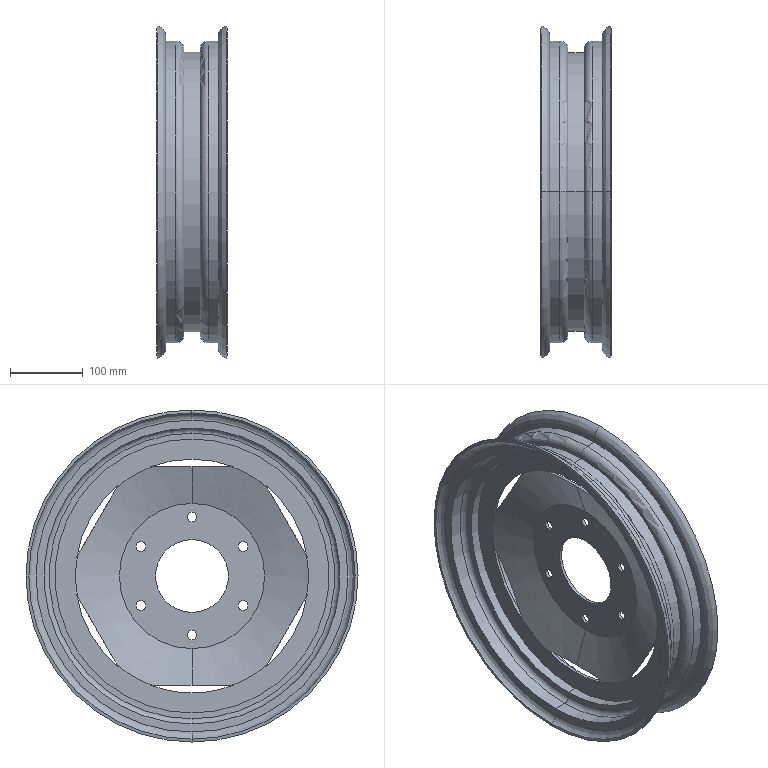Part | SolidWorks | 1 solid | 79 faces | box 96.667 x 455.608 x 455.608 mm | volume 1172743 mm3 | cylinder 35 | torus 18 | plane 18 | cone 8 | commonest cylinder face diameters 13.1 x12 320.649 x7 376 x4 406 x4 414 x4 100 x2